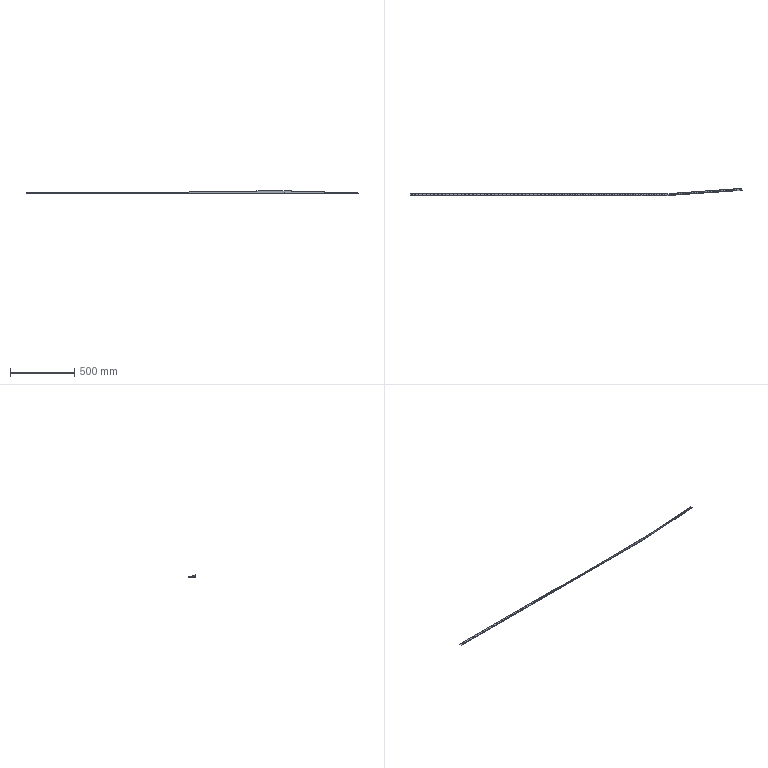Part | SolidWorks | features BaseBody 1 | 1 solid | 232 faces | box 2579 x 55.522 x 20.856 mm | volume 170207 mm3 | cylinder 220 | plane 12 | commonest cylinder face diameters 3.2 x220